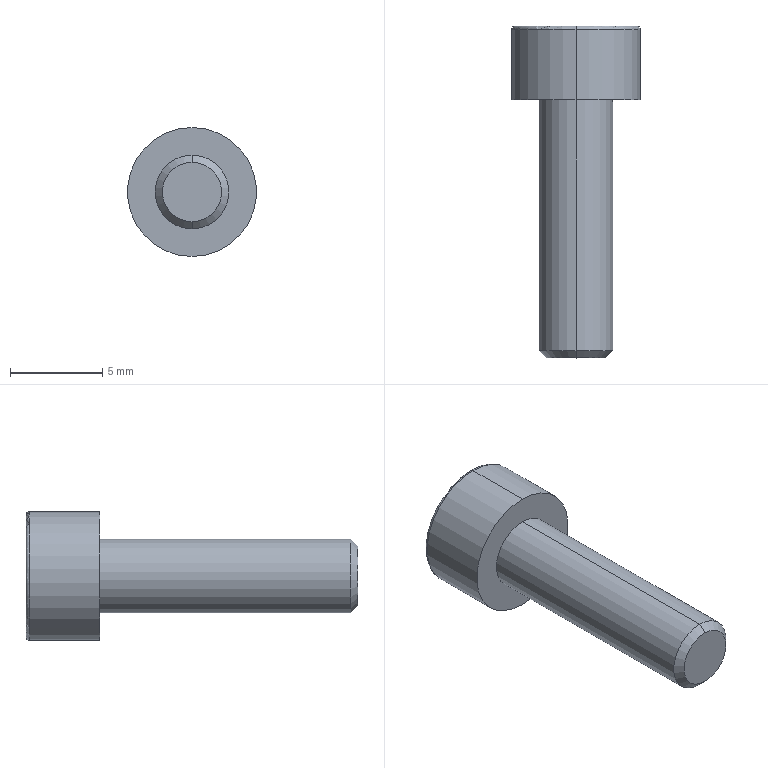Part | SolidWorks | features ICE 2, Chamfer 1, Extrusion 1, Fillet 1, RefAxis 1 | 1 solid | 18 faces | box 7 x 18 x 7 mm | volume 312.463 mm3 | plane 10 | cylinder 4 | cone 2 | torus 2 | commonest cylinder face diameters 4 x2 7 x2
STEP:
#1=CARTESIAN_POINT('',(0.,-14.,-1.61));
#2=VERTEX_POINT('',#1);
#3=CARTESIAN_POINT('',(0.,-14.,1.61));
#4=VERTEX_POINT('',#3);
#5=CARTESIAN_POINT('',(0.,-14.,0.));
#6=DIRECTION('',(0.,-1.,0.));
#7=DIRECTION('',(0.,0.,-1.));
#8=AXIS2_PLACEMENT_3D('',#5,#6,#7);
#9=CIRCLE('',#8,1.61);
#10=EDGE_CURVE('',#2,#4,#9,.T.);
#11=ORIENTED_EDGE('',*,*,#10,.F.);
#12=CARTESIAN_POINT('',(0.,-13.61,-2.));
#13=VERTEX_POINT('',#12);
#14=CARTESIAN_POINT('',(0.,-14.,-1.61));
#15=DIRECTION('',(0.,0.7071,-0.7071));
#16=VECTOR('',#15,1000.);
#17=LINE('',#14,#16);
#18=EDGE_CURVE('',#2,#13,#17,.T.);
#19=ORIENTED_EDGE('',*,*,#18,.T.);
#20=CARTESIAN_POINT('',(0.,-13.61,2.));
#21=VERTEX_POINT('',#20);
#22=CARTESIAN_POINT('',(0.,-13.61,0.));
#23=DIRECTION('',(0.,1.,0.));
#24=DIRECTION('',(0.,0.,-1.));
#25=AXIS2_PLACEMENT_3D('',#22,#23,#24);
#26=CIRCLE('',#25,2.);
#27=EDGE_CURVE('',#21,#13,#26,.T.);
#28=ORIENTED_EDGE('',*,*,#27,.F.);
#29=CARTESIAN_POINT('',(0.,-14.,1.61));
#30=DIRECTION('',(0.,0.7071,0.7071));
#31=VECTOR('',#30,1000.);
#32=LINE('',#29,#31);
#33=EDGE_CURVE('',#4,#21,#32,.T.);
#34=ORIENTED_EDGE('',*,*,#33,.F.);
#35=EDGE_LOOP('',(#11,#19,#28,#34));
#36=FACE_OUTER_BOUND('',#35,.T.);
#37=CARTESIAN_POINT('',(0.,-14.,0.));
#38=DIRECTION('',(0.,1.,0.));
#39=DIRECTION('',(0.,0.,1.));
#40=AXIS2_PLACEMENT_3D('',#37,#38,#39);
#41=CONICAL_SURFACE('',#40,1.61,0.7854);
#42=ADVANCED_FACE('',(#36),#41,.T.);
#43=ORIENTED_EDGE('',*,*,#27,.T.);
#44=CARTESIAN_POINT('',(0.,0.,-2.));
#45=VERTEX_POINT('',#44);
#46=CARTESIAN_POINT('',(0.,-14.,-2.));
#47=DIRECTION('',(0.,1.,0.));
#48=VECTOR('',#47,1000.);
#49=LINE('',#46,#48);
#50=EDGE_CURVE('',#13,#45,#49,.T.);
#51=ORIENTED_EDGE('',*,*,#50,.T.);
#52=CARTESIAN_POINT('',(0.,0.,2.));
#53=VERTEX_POINT('',#52);
#54=CARTESIAN_POINT('',(0.,0.,0.));
#55=DIRECTION('',(0.,-1.,0.));
#56=DIRECTION('',(0.,0.,1.));
#57=AXIS2_PLACEMENT_3D('',#54,#55,#56);
#58=CIRCLE('',#57,2.);
#59=EDGE_CURVE('',#45,#53,#58,.T.);
#60=ORIENTED_EDGE('',*,*,#59,.T.);
#61=CARTESIAN_POINT('',(0.,-14.,2.));
#62=DIRECTION('',(0.,1.,0.));
#63=VECTOR('',#62,1000.);
#64=LINE('',#61,#63);
#65=EDGE_CURVE('',#21,#53,#64,.T.);
#66=ORIENTED_EDGE('',*,*,#65,.F.);
#67=EDGE_LOOP('',(#43,#51,#60,#66));
#68=FACE_OUTER_BOUND('',#67,.T.);
#69=CARTESIAN_POINT('',(0.,-14.,0.));
#70=DIRECTION('',(0.,1.,0.));
#71=DIRECTION('',(0.,0.,1.));
#72=AXIS2_PLACEMENT_3D('',#69,#70,#71);
#73=CYLINDRICAL_SURFACE('',#72,2.);
#74=ADVANCED_FACE('',(#68),#73,.T.);
#75=CARTESIAN_POINT('',(0.,3.8,-3.5));
#76=VERTEX_POINT('',#75);
#77=CARTESIAN_POINT('',(0.,3.8,3.5));
#78=VERTEX_POINT('',#77);
#79=CARTESIAN_POINT('',(0.,3.8,0.));
#80=DIRECTION('',(0.,-1.,0.));
#81=DIRECTION('',(0.,0.,1.));
#82=AXIS2_PLACEMENT_3D('',#79,#80,#81);
#83=CIRCLE('',#82,3.5);
#84=EDGE_CURVE('',#76,#78,#83,.T.);
#85=ORIENTED_EDGE('',*,*,#84,.F.);
#86=CARTESIAN_POINT('',(0.,4.,-3.3));
#87=VERTEX_POINT('',#86);
#88=CARTESIAN_POINT('',(0.,3.8,-3.3));
#89=DIRECTION('',(1.,0.,0.));
#90=DIRECTION('',(0.,0.,-1.));
#91=AXIS2_PLACEMENT_3D('',#88,#89,#90);
#92=CIRCLE('',#91,0.2);
#93=EDGE_CURVE('',#76,#87,#92,.T.);
#94=ORIENTED_EDGE('',*,*,#93,.T.);
#95=CARTESIAN_POINT('',(0.,4.,3.3));
#96=VERTEX_POINT('',#95);
#97=CARTESIAN_POINT('',(0.,4.,0.));
#98=DIRECTION('',(0.,1.,0.));
#99=DIRECTION('',(0.,0.,1.));
#100=AXIS2_PLACEMENT_3D('',#97,#98,#99);
#101=CIRCLE('',#100,3.3);
#102=EDGE_CURVE('',#96,#87,#101,.T.);
#103=ORIENTED_EDGE('',*,*,#102,.F.);
#104=CARTESIAN_POINT('',(0.,3.8,3.3));
#105=DIRECTION('',(-1.,0.,0.));
#106=DIRECTION('',(0.,0.,1.));
#107=AXIS2_PLACEMENT_3D('',#104,#105,#106);
#108=CIRCLE('',#107,0.2);
#109=EDGE_CURVE('',#78,#96,#108,.T.);
#110=ORIENTED_EDGE('',*,*,#109,.F.);
#111=EDGE_LOOP('',(#85,#94,#103,#110));
#112=FACE_OUTER_BOUND('',#111,.T.);
#113=CARTESIAN_POINT('',(0.,3.8,0.));
#114=DIRECTION('',(0.,1.,0.));
#115=DIRECTION('',(0.,0.,1.));
#116=AXIS2_PLACEMENT_3D('',#113,#114,#115);
#117=TOROIDAL_SURFACE('',#116,3.3,0.2);
#118=ADVANCED_FACE('',(#112),#117,.T.);
#119=ORIENTED_EDGE('',*,*,#84,.T.);
#120=CARTESIAN_POINT('',(0.,0.,3.5));
#121=VERTEX_POINT('',#120);
#122=CARTESIAN_POINT('',(0.,4.,3.5));
#123=DIRECTION('',(0.,-1.,0.));
#124=VECTOR('',#123,1000.);
#125=LINE('',#122,#124);
#126=EDGE_CURVE('',#78,#121,#125,.T.);
#127=ORIENTED_EDGE('',*,*,#126,.T.);
#128=CARTESIAN_POINT('',(0.,0.,-3.5));
#129=VERTEX_POINT('',#128);
#130=CARTESIAN_POINT('',(0.,0.,0.));
#131=DIRECTION('',(0.,1.,0.));
#132=DIRECTION('',(0.,0.,1.));
#133=AXIS2_PLACEMENT_3D('',#130,#131,#132);
#134=CIRCLE('',#133,3.5);
#135=EDGE_CURVE('',#121,#129,#134,.T.);
#136=ORIENTED_EDGE('',*,*,#135,.T.);
#137=CARTESIAN_POINT('',(0.,4.,-3.5));
#138=DIRECTION('',(0.,-1.,0.));
#139=VECTOR('',#138,1000.);
#140=LINE('',#137,#139);
#141=EDGE_CURVE('',#76,#129,#140,.T.);
#142=ORIENTED_EDGE('',*,*,#141,.F.);
#143=EDGE_LOOP('',(#119,#127,#136,#142));
#144=FACE_OUTER_BOUND('',#143,.T.);
#145=CARTESIAN_POINT('',(0.,4.,0.));
#146=DIRECTION('',(0.,-1.,0.));
#147=DIRECTION('',(0.,0.,-1.));
#148=AXIS2_PLACEMENT_3D('',#145,#146,#147);
#149=CYLINDRICAL_SURFACE('',#148,3.5);
#150=ADVANCED_FACE('',(#144),#149,.T.);
#151=CARTESIAN_POINT('',(0.,0.,0.));
#152=DIRECTION('',(0.,1.,0.));
#153=DIRECTION('',(0.,0.,1.));
#154=AXIS2_PLACEMENT_3D('',#151,#152,#153);
#155=CIRCLE('',#154,3.5);
#156=EDGE_CURVE('',#129,#121,#155,.T.);
#157=ORIENTED_EDGE('',*,*,#156,.F.);
#158=ORIENTED_EDGE('',*,*,#135,.F.);
#159=EDGE_LOOP('',(#157,#158));
#160=FACE_OUTER_BOUND('',#159,.T.);
#161=CARTESIAN_POINT('',(0.,0.,0.));
#162=DIRECTION('',(0.,-1.,0.));
#163=DIRECTION('',(0.,0.,1.));
#164=AXIS2_PLACEMENT_3D('',#161,#162,#163);
#165=CIRCLE('',#164,2.);
#166=EDGE_CURVE('',#53,#45,#165,.T.);
#167=ORIENTED_EDGE('',*,*,#166,.F.);
#168=ORIENTED_EDGE('',*,*,#59,.F.);
#169=EDGE_LOOP('',(#167,#168));
#170=FACE_BOUND('',#169,.T.);
#171=CARTESIAN_POINT('',(0.,0.,0.));
#172=DIRECTION('',(0.,1.,0.));
#173=DIRECTION('',(0.,0.,1.));
#174=AXIS2_PLACEMENT_3D('',#171,#172,#173);
#175=PLANE('',#174);
#176=ADVANCED_FACE('',(#160,#170),#175,.F.);
#177=ORIENTED_EDGE('',*,*,#126,.F.);
#178=CARTESIAN_POINT('',(0.,3.8,0.));
#179=DIRECTION('',(0.,-1.,0.));
#180=DIRECTION('',(0.,0.,1.));
#181=AXIS2_PLACEMENT_3D('',#178,#179,#180);
#182=CIRCLE('',#181,3.5);
#183=EDGE_CURVE('',#78,#76,#182,.T.);
#184=ORIENTED_EDGE('',*,*,#183,.T.);
#185=ORIENTED_EDGE('',*,*,#141,.T.);
#186=ORIENTED_EDGE('',*,*,#156,.T.);
#187=EDGE_LOOP('',(#177,#184,#185,#186));
#188=FACE_OUTER_BOUND('',#187,.T.);
#189=CARTESIAN_POINT('',(0.,4.,0.));
#190=DIRECTION('',(0.,-1.,0.));
#191=DIRECTION('',(0.,0.,-1.));
#192=AXIS2_PLACEMENT_3D('',#189,#190,#191);
#193=CYLINDRICAL_SURFACE('',#192,3.5);
#194=ADVANCED_FACE('',(#188),#193,.T.);
#195=ORIENTED_EDGE('',*,*,#102,.T.);
#196=CARTESIAN_POINT('',(0.,4.,0.));
#197=DIRECTION('',(0.,1.,0.));
#198=DIRECTION('',(0.,0.,1.));
#199=AXIS2_PLACEMENT_3D('',#196,#197,#198);
#200=CIRCLE('',#199,3.3);
#201=EDGE_CURVE('',#87,#96,#200,.T.);
#202=ORIENTED_EDGE('',*,*,#201,.T.);
#203=EDGE_LOOP('',(#195,#202));
#204=FACE_OUTER_BOUND('',#203,.T.);
#205=CARTESIAN_POINT('',(0.8862,4.,1.535));
#206=VERTEX_POINT('',#205);
#207=CARTESIAN_POINT('',(1.772,4.,0.));
#208=VERTEX_POINT('',#207);
#209=CARTESIAN_POINT('',(0.8862,4.,1.535));
#210=DIRECTION('',(0.5,0.,-0.866));
#211=VECTOR('',#210,1000.);
#212=LINE('',#209,#211);
#213=EDGE_CURVE('',#206,#208,#212,.T.);
#214=ORIENTED_EDGE('',*,*,#213,.F.);
#215=CARTESIAN_POINT('',(-0.8862,4.,1.535));
#216=VERTEX_POINT('',#215);
#217=CARTESIAN_POINT('',(-0.8862,4.,1.535));
#218=DIRECTION('',(1.,0.,0.));
#219=VECTOR('',#218,1000.);
#220=LINE('',#217,#219);
#221=EDGE_CURVE('',#216,#206,#220,.T.);
#222=ORIENTED_EDGE('',*,*,#221,.F.);
#223=CARTESIAN_POINT('',(-1.772,4.,0.));
#224=VERTEX_POINT('',#223);
#225=CARTESIAN_POINT('',(-1.772,4.,0.));
#226=DIRECTION('',(0.5,0.,0.866));
#227=VECTOR('',#226,1000.);
#228=LINE('',#225,#227);
#229=EDGE_CURVE('',#224,#216,#228,.T.);
#230=ORIENTED_EDGE('',*,*,#229,.F.);
#231=CARTESIAN_POINT('',(-0.8862,4.,-1.535));
#232=VERTEX_POINT('',#231);
#233=CARTESIAN_POINT('',(-0.8862,4.,-1.535));
#234=DIRECTION('',(-0.5,0.,0.866));
#235=VECTOR('',#234,1000.);
#236=LINE('',#233,#235);
#237=EDGE_CURVE('',#232,#224,#236,.T.);
#238=ORIENTED_EDGE('',*,*,#237,.F.);
#239=CARTESIAN_POINT('',(0.8862,4.,-1.535));
#240=VERTEX_POINT('',#239);
#241=CARTESIAN_POINT('',(0.8862,4.,-1.535));
#242=DIRECTION('',(-1.,0.,0.));
#243=VECTOR('',#242,1000.);
#244=LINE('',#241,#243);
#245=EDGE_CURVE('',#240,#232,#244,.T.);
#246=ORIENTED_EDGE('',*,*,#245,.F.);
#247=CARTESIAN_POINT('',(1.772,4.,0.));
#248=DIRECTION('',(-0.5,0.,-0.866));
#249=VECTOR('',#248,1000.);
#250=LINE('',#247,#249);
#251=EDGE_CURVE('',#208,#240,#250,.T.);
#252=ORIENTED_EDGE('',*,*,#251,.F.);
#253=EDGE_LOOP('',(#214,#222,#230,#238,#246,#252));
#254=FACE_BOUND('',#253,.T.);
#255=CARTESIAN_POINT('',(0.,4.,0.));
#256=DIRECTION('',(0.,1.,0.));
#257=DIRECTION('',(0.,0.,1.));
#258=AXIS2_PLACEMENT_3D('',#255,#256,#257);
#259=PLANE('',#258);
#260=ADVANCED_FACE('',(#204,#254),#259,.T.);
#261=ORIENTED_EDGE('',*,*,#213,.T.);
#262=CARTESIAN_POINT('',(1.772,2.,0.));
#263=VERTEX_POINT('',#262);
#264=CARTESIAN_POINT('',(1.772,2.,0.));
#265=DIRECTION('',(0.,1.,0.));
#266=VECTOR('',#265,1000.);
#267=LINE('',#264,#266);
#268=EDGE_CURVE('',#263,#208,#267,.T.);
#269=ORIENTED_EDGE('',*,*,#268,.F.);
#270=CARTESIAN_POINT('',(0.8862,2.,1.535));
#271=VERTEX_POINT('',#270);
#272=CARTESIAN_POINT('',(0.8862,2.,1.535));
#273=DIRECTION('',(0.5,0.,-0.866));
#274=VECTOR('',#273,1000.);
#275=LINE('',#272,#274);
#276=EDGE_CURVE('',#271,#263,#275,.T.);
#277=ORIENTED_EDGE('',*,*,#276,.F.);
#278=CARTESIAN_POINT('',(0.8862,2.,1.535));
#279=DIRECTION('',(0.,1.,0.));
#280=VECTOR('',#279,1000.);
#281=LINE('',#278,#280);
#282=EDGE_CURVE('',#271,#206,#281,.T.);
#283=ORIENTED_EDGE('',*,*,#282,.T.);
#284=EDGE_LOOP('',(#261,#269,#277,#283));
#285=FACE_OUTER_BOUND('',#284,.T.);
#286=CARTESIAN_POINT('',(0.8862,2.,1.535));
#287=DIRECTION('',(0.866,0.,0.5));
#288=DIRECTION('',(0.5,0.,-0.866));
#289=AXIS2_PLACEMENT_3D('',#286,#287,#288);
#290=PLANE('',#289);
#291=ADVANCED_FACE('',(#285),#290,.F.);
#292=ORIENTED_EDGE('',*,*,#221,.T.);
#293=ORIENTED_EDGE('',*,*,#282,.F.);
#294=CARTESIAN_POINT('',(-0.8862,2.,1.535));
#295=VERTEX_POINT('',#294);
#296=CARTESIAN_POINT('',(-0.8862,2.,1.535));
#297=DIRECTION('',(1.,0.,0.));
#298=VECTOR('',#297,1000.);
#299=LINE('',#296,#298);
#300=EDGE_CURVE('',#295,#271,#299,.T.);
#301=ORIENTED_EDGE('',*,*,#300,.F.);
#302=CARTESIAN_POINT('',(-0.8862,2.,1.535));
#303=DIRECTION('',(0.,1.,0.));
#304=VECTOR('',#303,1000.);
#305=LINE('',#302,#304);
#306=EDGE_CURVE('',#295,#216,#305,.T.);
#307=ORIENTED_EDGE('',*,*,#306,.T.);
#308=EDGE_LOOP('',(#292,#293,#301,#307));
#309=FACE_OUTER_BOUND('',#308,.T.);
#310=CARTESIAN_POINT('',(-0.8862,2.,1.535));
#311=DIRECTION('',(0.,0.,1.));
#312=DIRECTION('',(1.,0.,0.));
#313=AXIS2_PLACEMENT_3D('',#310,#311,#312);
#314=PLANE('',#313);
#315=ADVANCED_FACE('',(#309),#314,.F.);
#316=ORIENTED_EDGE('',*,*,#229,.T.);
#317=ORIENTED_EDGE('',*,*,#306,.F.);
#318=CARTESIAN_POINT('',(-1.772,2.,0.));
#319=VERTEX_POINT('',#318);
#320=CARTESIAN_POINT('',(-1.772,2.,0.));
#321=DIRECTION('',(0.5,0.,0.866));
#322=VECTOR('',#321,1000.);
#323=LINE('',#320,#322);
#324=EDGE_CURVE('',#319,#295,#323,.T.);
#325=ORIENTED_EDGE('',*,*,#324,.F.);
#326=CARTESIAN_POINT('',(-1.772,2.,0.));
#327=DIRECTION('',(0.,1.,0.));
#328=VECTOR('',#327,1000.);
#329=LINE('',#326,#328);
#330=EDGE_CURVE('',#319,#224,#329,.T.);
#331=ORIENTED_EDGE('',*,*,#330,.T.);
#332=EDGE_LOOP('',(#316,#317,#325,#331));
#333=FACE_OUTER_BOUND('',#332,.T.);
#334=CARTESIAN_POINT('',(-1.772,2.,0.));
#335=DIRECTION('',(-0.866,0.,0.5));
#336=DIRECTION('',(0.5,0.,0.866));
#337=AXIS2_PLACEMENT_3D('',#334,#335,#336);
#338=PLANE('',#337);
#339=ADVANCED_FACE('',(#333),#338,.F.);
#340=ORIENTED_EDGE('',*,*,#237,.T.);
#341=ORIENTED_EDGE('',*,*,#330,.F.);
#342=CARTESIAN_POINT('',(-0.8862,2.,-1.535));
#343=VERTEX_POINT('',#342);
#344=CARTESIAN_POINT('',(-0.8862,2.,-1.535));
#345=DIRECTION('',(-0.5,0.,0.866));
#346=VECTOR('',#345,1000.);
#347=LINE('',#344,#346);
#348=EDGE_CURVE('',#343,#319,#347,.T.);
#349=ORIENTED_EDGE('',*,*,#348,.F.);
#350=CARTESIAN_POINT('',(-0.8862,2.,-1.535));
#351=DIRECTION('',(0.,1.,0.));
#352=VECTOR('',#351,1000.);
#353=LINE('',#350,#352);
#354=EDGE_CURVE('',#343,#232,#353,.T.);
#355=ORIENTED_EDGE('',*,*,#354,.T.);
#356=EDGE_LOOP('',(#340,#341,#349,#355));
#357=FACE_OUTER_BOUND('',#356,.T.);
#358=CARTESIAN_POINT('',(-0.8862,2.,-1.535));
#359=DIRECTION('',(-0.866,0.,-0.5));
#360=DIRECTION('',(-0.5,0.,0.866));
#361=AXIS2_PLACEMENT_3D('',#358,#359,#360);
#362=PLANE('',#361);
#363=ADVANCED_FACE('',(#357),#362,.F.);
#364=ORIENTED_EDGE('',*,*,#245,.T.);
#365=ORIENTED_EDGE('',*,*,#354,.F.);
#366=CARTESIAN_POINT('',(0.8862,2.,-1.535));
#367=VERTEX_POINT('',#366);
#368=CARTESIAN_POINT('',(0.8862,2.,-1.535));
#369=DIRECTION('',(-1.,0.,0.));
#370=VECTOR('',#369,1000.);
#371=LINE('',#368,#370);
#372=EDGE_CURVE('',#367,#343,#371,.T.);
#373=ORIENTED_EDGE('',*,*,#372,.F.);
#374=CARTESIAN_POINT('',(0.8862,2.,-1.535));
#375=DIRECTION('',(0.,1.,0.));
#376=VECTOR('',#375,1000.);
#377=LINE('',#374,#376);
#378=EDGE_CURVE('',#367,#240,#377,.T.);
#379=ORIENTED_EDGE('',*,*,#378,.T.);
#380=EDGE_LOOP('',(#364,#365,#373,#379));
#381=FACE_OUTER_BOUND('',#380,.T.);
#382=CARTESIAN_POINT('',(0.8862,2.,-1.535));
#383=DIRECTION('',(0.,0.,-1.));
#384=DIRECTION('',(-1.,0.,0.));
#385=AXIS2_PLACEMENT_3D('',#382,#383,#384);
#386=PLANE('',#385);
#387=ADVANCED_FACE('',(#381),#386,.F.);
#388=ORIENTED_EDGE('',*,*,#251,.T.);
#389=ORIENTED_EDGE('',*,*,#378,.F.);
#390=CARTESIAN_POINT('',(1.772,2.,0.));
#391=DIRECTION('',(-0.5,0.,-0.866));
#392=VECTOR('',#391,1000.);
#393=LINE('',#390,#392);
#394=EDGE_CURVE('',#263,#367,#393,.T.);
#395=ORIENTED_EDGE('',*,*,#394,.F.);
#396=ORIENTED_EDGE('',*,*,#268,.T.);
#397=EDGE_LOOP('',(#388,#389,#395,#396));
#398=FACE_OUTER_BOUND('',#397,.T.);
#399=CARTESIAN_POINT('',(1.772,2.,0.));
#400=DIRECTION('',(0.866,0.,-0.5));
#401=DIRECTION('',(-0.5,0.,-0.866));
#402=AXIS2_PLACEMENT_3D('',#399,#400,#401);
#403=PLANE('',#402);
#404=ADVANCED_FACE('',(#398),#403,.F.);
#405=ORIENTED_EDGE('',*,*,#276,.T.);
#406=ORIENTED_EDGE('',*,*,#394,.T.);
#407=ORIENTED_EDGE('',*,*,#372,.T.);
#408=ORIENTED_EDGE('',*,*,#348,.T.);
#409=ORIENTED_EDGE('',*,*,#324,.T.);
#410=ORIENTED_EDGE('',*,*,#300,.T.);
#411=EDGE_LOOP('',(#405,#406,#407,#408,#409,#410));
#412=FACE_OUTER_BOUND('',#411,.T.);
#413=CARTESIAN_POINT('',(0.,2.,0.));
#414=DIRECTION('',(0.,1.,0.));
#415=DIRECTION('',(0.,0.,1.));
#416=AXIS2_PLACEMENT_3D('',#413,#414,#415);
#417=PLANE('',#416);
#418=ADVANCED_FACE('',(#412),#417,.T.);
#419=ORIENTED_EDGE('',*,*,#93,.F.);
#420=ORIENTED_EDGE('',*,*,#183,.F.);
#421=ORIENTED_EDGE('',*,*,#109,.T.);
#422=ORIENTED_EDGE('',*,*,#201,.F.);
#423=EDGE_LOOP('',(#419,#420,#421,#422));
#424=FACE_OUTER_BOUND('',#423,.T.);
#425=CARTESIAN_POINT('',(0.,3.8,0.));
#426=DIRECTION('',(0.,1.,0.));
#427=DIRECTION('',(0.,0.,1.));
#428=AXIS2_PLACEMENT_3D('',#425,#426,#427);
#429=TOROIDAL_SURFACE('',#428,3.3,0.2);
#430=ADVANCED_FACE('',(#424),#429,.T.);
#431=ORIENTED_EDGE('',*,*,#50,.F.);
#432=CARTESIAN_POINT('',(0.,-13.61,0.));
#433=DIRECTION('',(0.,1.,0.));
#434=DIRECTION('',(0.,0.,-1.));
#435=AXIS2_PLACEMENT_3D('',#432,#433,#434);
#436=CIRCLE('',#435,2.);
#437=EDGE_CURVE('',#13,#21,#436,.T.);
#438=ORIENTED_EDGE('',*,*,#437,.T.);
#439=ORIENTED_EDGE('',*,*,#65,.T.);
#440=ORIENTED_EDGE('',*,*,#166,.T.);
#441=EDGE_LOOP('',(#431,#438,#439,#440));
#442=FACE_OUTER_BOUND('',#441,.T.);
#443=CARTESIAN_POINT('',(0.,-14.,0.));
#444=DIRECTION('',(0.,1.,0.));
#445=DIRECTION('',(0.,0.,1.));
#446=AXIS2_PLACEMENT_3D('',#443,#444,#445);
#447=CYLINDRICAL_SURFACE('',#446,2.);
#448=ADVANCED_FACE('',(#442),#447,.T.);
#449=CARTESIAN_POINT('',(0.,-14.,0.));
#450=DIRECTION('',(0.,-1.,0.));
#451=DIRECTION('',(0.,0.,-1.));
#452=AXIS2_PLACEMENT_3D('',#449,#450,#451);
#453=CIRCLE('',#452,1.61);
#454=EDGE_CURVE('',#4,#2,#453,.T.);
#455=ORIENTED_EDGE('',*,*,#454,.T.);
#456=ORIENTED_EDGE('',*,*,#10,.T.);
#457=EDGE_LOOP('',(#455,#456));
#458=FACE_OUTER_BOUND('',#457,.T.);
#459=CARTESIAN_POINT('',(0.,-14.,0.));
#460=DIRECTION('',(0.,-1.,0.));
#461=DIRECTION('',(0.,0.,-1.));
#462=AXIS2_PLACEMENT_3D('',#459,#460,#461);
#463=PLANE('',#462);
#464=ADVANCED_FACE('',(#458),#463,.T.);
#465=ORIENTED_EDGE('',*,*,#18,.F.);
#466=ORIENTED_EDGE('',*,*,#454,.F.);
#467=ORIENTED_EDGE('',*,*,#33,.T.);
#468=ORIENTED_EDGE('',*,*,#437,.F.);
#469=EDGE_LOOP('',(#465,#466,#467,#468));
#470=FACE_OUTER_BOUND('',#469,.T.);
#471=CARTESIAN_POINT('',(0.,-14.,0.));
#472=DIRECTION('',(0.,1.,0.));
#473=DIRECTION('',(0.,0.,1.));
#474=AXIS2_PLACEMENT_3D('',#471,#472,#473);
#475=CONICAL_SURFACE('',#474,1.61,0.7854);
#476=ADVANCED_FACE('',(#470),#475,.T.);
#477=CLOSED_SHELL('',(#42,#74,#118,#150,#176,#194,#260,#291,#315,#339,#363,#387,#404,#418,#430,#448,#464,#476));
#478=MANIFOLD_SOLID_BREP('',#477);
#479=CARTESIAN_POINT('',(0.,0.,0.));
#480=DIRECTION('',(0.,0.,1.));
#481=DIRECTION('',(1.,0.,0.));
#482=AXIS2_PLACEMENT_3D('',#479,#480,#481);
#483=(LENGTH_UNIT()NAMED_UNIT(*)SI_UNIT(.MILLI.,.METRE.));
#484=UNCERTAINTY_MEASURE_WITH_UNIT(LENGTH_MEASURE(0.00001),#483,'','');
#485=(NAMED_UNIT(*)PLANE_ANGLE_UNIT()SI_UNIT($,.RADIAN.));
#486=(NAMED_UNIT(*)SI_UNIT($,.STERADIAN.)SOLID_ANGLE_UNIT());
#487=(GEOMETRIC_REPRESENTATION_CONTEXT(3)GLOBAL_UNCERTAINTY_ASSIGNED_CONTEXT((#484))GLOBAL_UNIT_ASSIGNED_CONTEXT((#483,#485,#486))REPRESENTATION_CONTEXT('',''));
#488=ADVANCED_BREP_SHAPE_REPRESENTATION('',(#478,#482),#487);